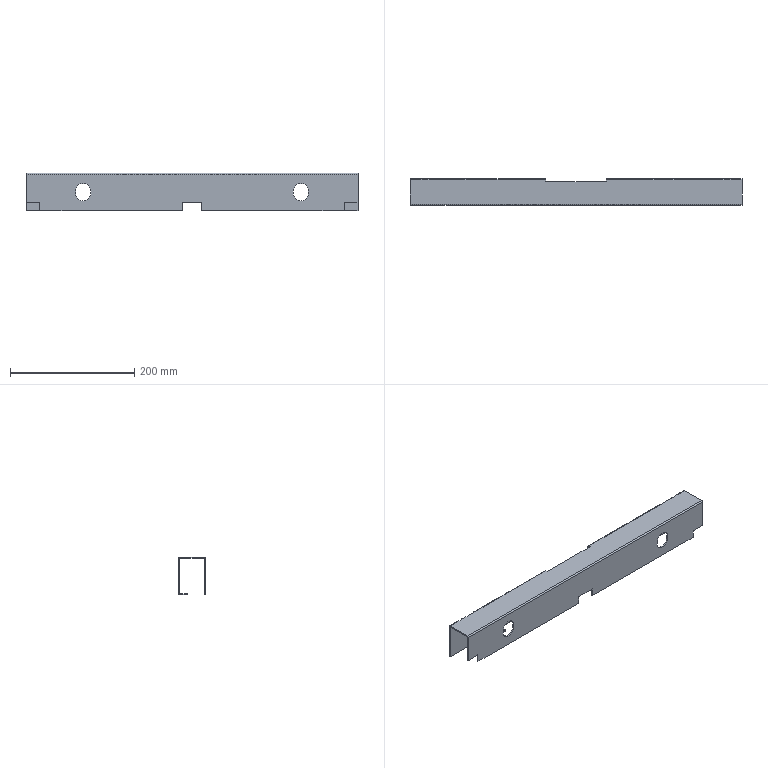Part | NX | features solid 2 | 1 solid | 149 faces | box 534 x 43.2 x 60.503 mm | volume 143631 mm3 | plane 110 | cylinder 33 | spline 6 | commonest cylinder face diameters 4 x9 2 x4 6 x4 14 x4 24 x4 43 x4